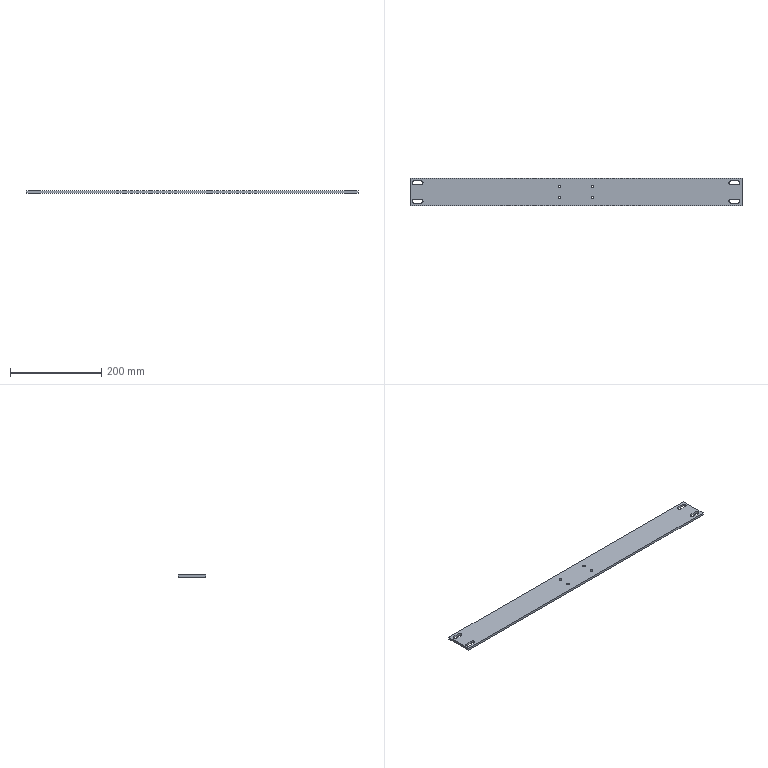Part | STEP file | 1 solid | 34 faces | box 726 x 60 x 5 mm | volume 213262 mm3 | cylinder 20 | plane 14 | commonest cylinder face diameters 9 x12 6 x8